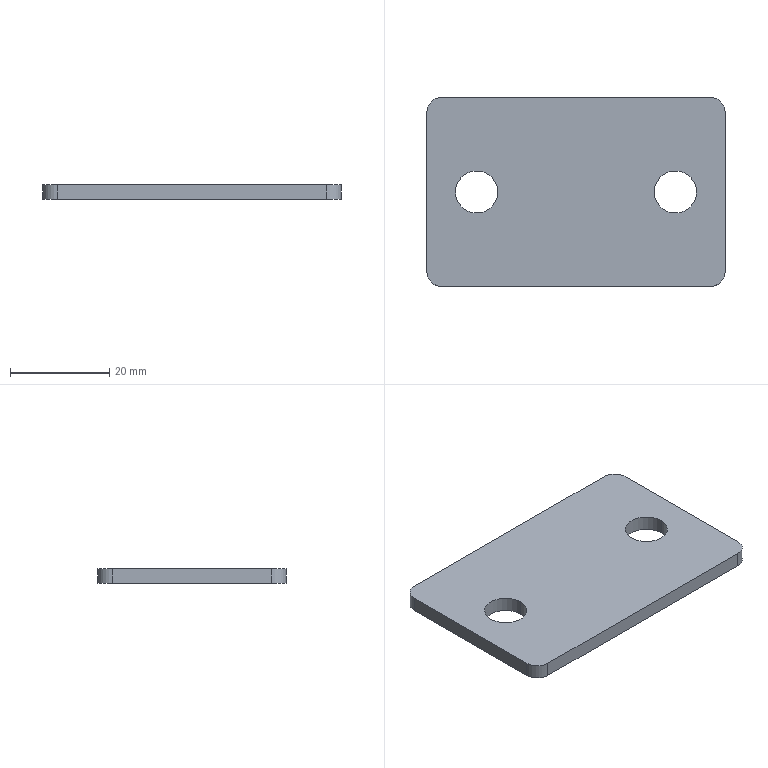Part | SolidWorks | features BaseBody 1 | 1 solid | 14 faces | box 60 x 38 x 3 mm | volume 6476 mm3 | cylinder 8 | plane 6 | commonest cylinder face diameters 6 x4 8.5 x4
STEP:
#1=CARTESIAN_POINT('',(54.25,0.,0.));
#2=VERTEX_POINT('',#1);
#3=CARTESIAN_POINT('',(45.75,0.,0.));
#4=VERTEX_POINT('',#3);
#5=CARTESIAN_POINT('',(50.,0.,0.));
#6=DIRECTION('',(0.,0.,-1.));
#7=DIRECTION('',(-1.,0.,0.));
#8=AXIS2_PLACEMENT_3D('',#5,#6,#7);
#9=CIRCLE('',#8,4.25);
#10=EDGE_CURVE('',#2,#4,#9,.T.);
#11=ORIENTED_EDGE('',*,*,#10,.F.);
#12=CARTESIAN_POINT('',(54.25,0.,-3.));
#13=VERTEX_POINT('',#12);
#14=CARTESIAN_POINT('',(54.25,0.,-3.));
#15=DIRECTION('',(0.,0.,-1.));
#16=VECTOR('',#15,1000.);
#17=LINE('',#14,#16);
#18=EDGE_CURVE('',#2,#13,#17,.T.);
#19=ORIENTED_EDGE('',*,*,#18,.T.);
#20=CARTESIAN_POINT('',(45.75,0.,-3.));
#21=VERTEX_POINT('',#20);
#22=CARTESIAN_POINT('',(50.,0.,-3.));
#23=DIRECTION('',(0.,0.,-1.));
#24=DIRECTION('',(-1.,0.,0.));
#25=AXIS2_PLACEMENT_3D('',#22,#23,#24);
#26=CIRCLE('',#25,4.25);
#27=EDGE_CURVE('',#13,#21,#26,.T.);
#28=ORIENTED_EDGE('',*,*,#27,.T.);
#29=CARTESIAN_POINT('',(45.75,0.,-3.));
#30=DIRECTION('',(0.,0.,-1.));
#31=VECTOR('',#30,1000.);
#32=LINE('',#29,#31);
#33=EDGE_CURVE('',#4,#21,#32,.T.);
#34=ORIENTED_EDGE('',*,*,#33,.F.);
#35=EDGE_LOOP('',(#11,#19,#28,#34));
#36=FACE_OUTER_BOUND('',#35,.T.);
#37=CARTESIAN_POINT('',(50.,0.,-3.));
#38=DIRECTION('',(0.,0.,-1.));
#39=DIRECTION('',(-1.,0.,0.));
#40=AXIS2_PLACEMENT_3D('',#37,#38,#39);
#41=CYLINDRICAL_SURFACE('',#40,4.25);
#42=ADVANCED_FACE('',(#36),#41,.F.);
#43=CARTESIAN_POINT('',(14.25,0.,0.));
#44=VERTEX_POINT('',#43);
#45=CARTESIAN_POINT('',(5.75,0.,0.));
#46=VERTEX_POINT('',#45);
#47=CARTESIAN_POINT('',(10.,0.,0.));
#48=DIRECTION('',(0.,0.,-1.));
#49=DIRECTION('',(-1.,0.,0.));
#50=AXIS2_PLACEMENT_3D('',#47,#48,#49);
#51=CIRCLE('',#50,4.25);
#52=EDGE_CURVE('',#44,#46,#51,.T.);
#53=ORIENTED_EDGE('',*,*,#52,.F.);
#54=CARTESIAN_POINT('',(14.25,0.,-3.));
#55=VERTEX_POINT('',#54);
#56=CARTESIAN_POINT('',(14.25,0.,-3.));
#57=DIRECTION('',(0.,0.,-1.));
#58=VECTOR('',#57,1000.);
#59=LINE('',#56,#58);
#60=EDGE_CURVE('',#44,#55,#59,.T.);
#61=ORIENTED_EDGE('',*,*,#60,.T.);
#62=CARTESIAN_POINT('',(5.75,0.,-3.));
#63=VERTEX_POINT('',#62);
#64=CARTESIAN_POINT('',(10.,0.,-3.));
#65=DIRECTION('',(0.,0.,-1.));
#66=DIRECTION('',(-1.,0.,0.));
#67=AXIS2_PLACEMENT_3D('',#64,#65,#66);
#68=CIRCLE('',#67,4.25);
#69=EDGE_CURVE('',#55,#63,#68,.T.);
#70=ORIENTED_EDGE('',*,*,#69,.T.);
#71=CARTESIAN_POINT('',(5.75,0.,-3.));
#72=DIRECTION('',(0.,0.,-1.));
#73=VECTOR('',#72,1000.);
#74=LINE('',#71,#73);
#75=EDGE_CURVE('',#46,#63,#74,.T.);
#76=ORIENTED_EDGE('',*,*,#75,.F.);
#77=EDGE_LOOP('',(#53,#61,#70,#76));
#78=FACE_OUTER_BOUND('',#77,.T.);
#79=CARTESIAN_POINT('',(10.,0.,-3.));
#80=DIRECTION('',(0.,0.,-1.));
#81=DIRECTION('',(-1.,0.,0.));
#82=AXIS2_PLACEMENT_3D('',#79,#80,#81);
#83=CYLINDRICAL_SURFACE('',#82,4.25);
#84=ADVANCED_FACE('',(#78),#83,.F.);
#85=CARTESIAN_POINT('',(57.,19.,-3.));
#86=VERTEX_POINT('',#85);
#87=CARTESIAN_POINT('',(3.,19.,-3.));
#88=VERTEX_POINT('',#87);
#89=CARTESIAN_POINT('',(3.,19.,-3.));
#90=DIRECTION('',(-1.,0.,0.));
#91=VECTOR('',#90,1000.);
#92=LINE('',#89,#91);
#93=EDGE_CURVE('',#86,#88,#92,.T.);
#94=ORIENTED_EDGE('',*,*,#93,.F.);
#95=CARTESIAN_POINT('',(60.,16.,-3.));
#96=VERTEX_POINT('',#95);
#97=CARTESIAN_POINT('',(57.,16.,-3.));
#98=DIRECTION('',(0.,0.,1.));
#99=DIRECTION('',(-1.,0.,0.));
#100=AXIS2_PLACEMENT_3D('',#97,#98,#99);
#101=CIRCLE('',#100,3.);
#102=EDGE_CURVE('',#96,#86,#101,.T.);
#103=ORIENTED_EDGE('',*,*,#102,.F.);
#104=CARTESIAN_POINT('',(60.,-16.,-3.));
#105=VERTEX_POINT('',#104);
#106=CARTESIAN_POINT('',(60.,16.,-3.));
#107=DIRECTION('',(0.,1.,0.));
#108=VECTOR('',#107,1000.);
#109=LINE('',#106,#108);
#110=EDGE_CURVE('',#105,#96,#109,.T.);
#111=ORIENTED_EDGE('',*,*,#110,.F.);
#112=CARTESIAN_POINT('',(57.,-19.,-3.));
#113=VERTEX_POINT('',#112);
#114=CARTESIAN_POINT('',(57.,-16.,-3.));
#115=DIRECTION('',(0.,0.,1.));
#116=DIRECTION('',(-1.,0.,0.));
#117=AXIS2_PLACEMENT_3D('',#114,#115,#116);
#118=CIRCLE('',#117,3.);
#119=EDGE_CURVE('',#113,#105,#118,.T.);
#120=ORIENTED_EDGE('',*,*,#119,.F.);
#121=CARTESIAN_POINT('',(3.,-19.,-3.));
#122=VERTEX_POINT('',#121);
#123=CARTESIAN_POINT('',(3.,-19.,-3.));
#124=DIRECTION('',(1.,0.,0.));
#125=VECTOR('',#124,1000.);
#126=LINE('',#123,#125);
#127=EDGE_CURVE('',#122,#113,#126,.T.);
#128=ORIENTED_EDGE('',*,*,#127,.F.);
#129=CARTESIAN_POINT('',(0.,-16.,-3.));
#130=VERTEX_POINT('',#129);
#131=CARTESIAN_POINT('',(3.,-16.,-3.));
#132=DIRECTION('',(0.,0.,1.));
#133=DIRECTION('',(-1.,0.,0.));
#134=AXIS2_PLACEMENT_3D('',#131,#132,#133);
#135=CIRCLE('',#134,3.);
#136=EDGE_CURVE('',#130,#122,#135,.T.);
#137=ORIENTED_EDGE('',*,*,#136,.F.);
#138=CARTESIAN_POINT('',(0.,16.,-3.));
#139=VERTEX_POINT('',#138);
#140=CARTESIAN_POINT('',(0.,16.,-3.));
#141=DIRECTION('',(0.,-1.,0.));
#142=VECTOR('',#141,1000.);
#143=LINE('',#140,#142);
#144=EDGE_CURVE('',#139,#130,#143,.T.);
#145=ORIENTED_EDGE('',*,*,#144,.F.);
#146=CARTESIAN_POINT('',(3.,16.,-3.));
#147=DIRECTION('',(0.,0.,1.));
#148=DIRECTION('',(-1.,0.,0.));
#149=AXIS2_PLACEMENT_3D('',#146,#147,#148);
#150=CIRCLE('',#149,3.);
#151=EDGE_CURVE('',#88,#139,#150,.T.);
#152=ORIENTED_EDGE('',*,*,#151,.F.);
#153=EDGE_LOOP('',(#94,#103,#111,#120,#128,#137,#145,#152));
#154=FACE_OUTER_BOUND('',#153,.T.);
#155=CARTESIAN_POINT('',(50.,0.,-3.));
#156=DIRECTION('',(0.,0.,-1.));
#157=DIRECTION('',(-1.,0.,0.));
#158=AXIS2_PLACEMENT_3D('',#155,#156,#157);
#159=CIRCLE('',#158,4.25);
#160=EDGE_CURVE('',#21,#13,#159,.T.);
#161=ORIENTED_EDGE('',*,*,#160,.F.);
#162=ORIENTED_EDGE('',*,*,#27,.F.);
#163=EDGE_LOOP('',(#161,#162));
#164=FACE_BOUND('',#163,.T.);
#165=CARTESIAN_POINT('',(10.,0.,-3.));
#166=DIRECTION('',(0.,0.,-1.));
#167=DIRECTION('',(-1.,0.,0.));
#168=AXIS2_PLACEMENT_3D('',#165,#166,#167);
#169=CIRCLE('',#168,4.25);
#170=EDGE_CURVE('',#63,#55,#169,.T.);
#171=ORIENTED_EDGE('',*,*,#170,.F.);
#172=ORIENTED_EDGE('',*,*,#69,.F.);
#173=EDGE_LOOP('',(#171,#172));
#174=FACE_BOUND('',#173,.T.);
#175=CARTESIAN_POINT('',(3.,16.,-3.));
#176=DIRECTION('',(0.,0.,1.));
#177=DIRECTION('',(1.,0.,0.));
#178=AXIS2_PLACEMENT_3D('',#175,#176,#177);
#179=PLANE('',#178);
#180=ADVANCED_FACE('',(#154,#164,#174),#179,.F.);
#181=ORIENTED_EDGE('',*,*,#151,.T.);
#182=CARTESIAN_POINT('',(0.,16.,0.));
#183=VERTEX_POINT('',#182);
#184=CARTESIAN_POINT('',(0.,16.,-3.));
#185=DIRECTION('',(0.,0.,1.));
#186=VECTOR('',#185,1000.);
#187=LINE('',#184,#186);
#188=EDGE_CURVE('',#139,#183,#187,.T.);
#189=ORIENTED_EDGE('',*,*,#188,.T.);
#190=CARTESIAN_POINT('',(3.,19.,0.));
#191=VERTEX_POINT('',#190);
#192=CARTESIAN_POINT('',(3.,16.,0.));
#193=DIRECTION('',(0.,0.,-1.));
#194=DIRECTION('',(-1.,0.,0.));
#195=AXIS2_PLACEMENT_3D('',#192,#193,#194);
#196=CIRCLE('',#195,3.);
#197=EDGE_CURVE('',#183,#191,#196,.T.);
#198=ORIENTED_EDGE('',*,*,#197,.T.);
#199=CARTESIAN_POINT('',(3.,19.,-3.));
#200=DIRECTION('',(0.,0.,-1.));
#201=VECTOR('',#200,1000.);
#202=LINE('',#199,#201);
#203=EDGE_CURVE('',#191,#88,#202,.T.);
#204=ORIENTED_EDGE('',*,*,#203,.T.);
#205=EDGE_LOOP('',(#181,#189,#198,#204));
#206=FACE_OUTER_BOUND('',#205,.T.);
#207=CARTESIAN_POINT('',(3.,16.,-3.));
#208=DIRECTION('',(0.,0.,-1.));
#209=DIRECTION('',(-1.,0.,0.));
#210=AXIS2_PLACEMENT_3D('',#207,#208,#209);
#211=CYLINDRICAL_SURFACE('',#210,3.);
#212=ADVANCED_FACE('',(#206),#211,.T.);
#213=ORIENTED_EDGE('',*,*,#93,.T.);
#214=ORIENTED_EDGE('',*,*,#203,.F.);
#215=CARTESIAN_POINT('',(57.,19.,0.));
#216=VERTEX_POINT('',#215);
#217=CARTESIAN_POINT('',(57.,19.,0.));
#218=DIRECTION('',(1.,0.,0.));
#219=VECTOR('',#218,1000.);
#220=LINE('',#217,#219);
#221=EDGE_CURVE('',#191,#216,#220,.T.);
#222=ORIENTED_EDGE('',*,*,#221,.T.);
#223=CARTESIAN_POINT('',(57.,19.,-3.));
#224=DIRECTION('',(0.,0.,-1.));
#225=VECTOR('',#224,1000.);
#226=LINE('',#223,#225);
#227=EDGE_CURVE('',#216,#86,#226,.T.);
#228=ORIENTED_EDGE('',*,*,#227,.T.);
#229=EDGE_LOOP('',(#213,#214,#222,#228));
#230=FACE_OUTER_BOUND('',#229,.T.);
#231=CARTESIAN_POINT('',(57.,19.,-3.));
#232=DIRECTION('',(0.,1.,0.));
#233=DIRECTION('',(0.,0.,1.));
#234=AXIS2_PLACEMENT_3D('',#231,#232,#233);
#235=PLANE('',#234);
#236=ADVANCED_FACE('',(#230),#235,.T.);
#237=ORIENTED_EDGE('',*,*,#102,.T.);
#238=ORIENTED_EDGE('',*,*,#227,.F.);
#239=CARTESIAN_POINT('',(60.,16.,0.));
#240=VERTEX_POINT('',#239);
#241=CARTESIAN_POINT('',(57.,16.,0.));
#242=DIRECTION('',(0.,0.,-1.));
#243=DIRECTION('',(-1.,0.,0.));
#244=AXIS2_PLACEMENT_3D('',#241,#242,#243);
#245=CIRCLE('',#244,3.);
#246=EDGE_CURVE('',#216,#240,#245,.T.);
#247=ORIENTED_EDGE('',*,*,#246,.T.);
#248=CARTESIAN_POINT('',(60.,16.,-3.));
#249=DIRECTION('',(0.,0.,-1.));
#250=VECTOR('',#249,1000.);
#251=LINE('',#248,#250);
#252=EDGE_CURVE('',#240,#96,#251,.T.);
#253=ORIENTED_EDGE('',*,*,#252,.T.);
#254=EDGE_LOOP('',(#237,#238,#247,#253));
#255=FACE_OUTER_BOUND('',#254,.T.);
#256=CARTESIAN_POINT('',(57.,16.,-3.));
#257=DIRECTION('',(0.,0.,-1.));
#258=DIRECTION('',(-1.,0.,0.));
#259=AXIS2_PLACEMENT_3D('',#256,#257,#258);
#260=CYLINDRICAL_SURFACE('',#259,3.);
#261=ADVANCED_FACE('',(#255),#260,.T.);
#262=ORIENTED_EDGE('',*,*,#110,.T.);
#263=ORIENTED_EDGE('',*,*,#252,.F.);
#264=CARTESIAN_POINT('',(60.,-16.,0.));
#265=VERTEX_POINT('',#264);
#266=CARTESIAN_POINT('',(60.,-16.,0.));
#267=DIRECTION('',(0.,-1.,0.));
#268=VECTOR('',#267,1000.);
#269=LINE('',#266,#268);
#270=EDGE_CURVE('',#240,#265,#269,.T.);
#271=ORIENTED_EDGE('',*,*,#270,.T.);
#272=CARTESIAN_POINT('',(60.,-16.,-3.));
#273=DIRECTION('',(0.,0.,-1.));
#274=VECTOR('',#273,1000.);
#275=LINE('',#272,#274);
#276=EDGE_CURVE('',#265,#105,#275,.T.);
#277=ORIENTED_EDGE('',*,*,#276,.T.);
#278=EDGE_LOOP('',(#262,#263,#271,#277));
#279=FACE_OUTER_BOUND('',#278,.T.);
#280=CARTESIAN_POINT('',(60.,-16.,-3.));
#281=DIRECTION('',(1.,0.,0.));
#282=DIRECTION('',(0.,0.,-1.));
#283=AXIS2_PLACEMENT_3D('',#280,#281,#282);
#284=PLANE('',#283);
#285=ADVANCED_FACE('',(#279),#284,.T.);
#286=ORIENTED_EDGE('',*,*,#119,.T.);
#287=ORIENTED_EDGE('',*,*,#276,.F.);
#288=CARTESIAN_POINT('',(57.,-19.,0.));
#289=VERTEX_POINT('',#288);
#290=CARTESIAN_POINT('',(57.,-16.,0.));
#291=DIRECTION('',(0.,0.,-1.));
#292=DIRECTION('',(-1.,0.,0.));
#293=AXIS2_PLACEMENT_3D('',#290,#291,#292);
#294=CIRCLE('',#293,3.);
#295=EDGE_CURVE('',#265,#289,#294,.T.);
#296=ORIENTED_EDGE('',*,*,#295,.T.);
#297=CARTESIAN_POINT('',(57.,-19.,-3.));
#298=DIRECTION('',(0.,0.,-1.));
#299=VECTOR('',#298,1000.);
#300=LINE('',#297,#299);
#301=EDGE_CURVE('',#289,#113,#300,.T.);
#302=ORIENTED_EDGE('',*,*,#301,.T.);
#303=EDGE_LOOP('',(#286,#287,#296,#302));
#304=FACE_OUTER_BOUND('',#303,.T.);
#305=CARTESIAN_POINT('',(57.,-16.,-3.));
#306=DIRECTION('',(0.,0.,-1.));
#307=DIRECTION('',(-1.,0.,0.));
#308=AXIS2_PLACEMENT_3D('',#305,#306,#307);
#309=CYLINDRICAL_SURFACE('',#308,3.);
#310=ADVANCED_FACE('',(#304),#309,.T.);
#311=ORIENTED_EDGE('',*,*,#127,.T.);
#312=ORIENTED_EDGE('',*,*,#301,.F.);
#313=CARTESIAN_POINT('',(3.,-19.,0.));
#314=VERTEX_POINT('',#313);
#315=CARTESIAN_POINT('',(3.,-19.,0.));
#316=DIRECTION('',(-1.,0.,0.));
#317=VECTOR('',#316,1000.);
#318=LINE('',#315,#317);
#319=EDGE_CURVE('',#289,#314,#318,.T.);
#320=ORIENTED_EDGE('',*,*,#319,.T.);
#321=CARTESIAN_POINT('',(3.,-19.,-3.));
#322=DIRECTION('',(0.,0.,-1.));
#323=VECTOR('',#322,1000.);
#324=LINE('',#321,#323);
#325=EDGE_CURVE('',#314,#122,#324,.T.);
#326=ORIENTED_EDGE('',*,*,#325,.T.);
#327=EDGE_LOOP('',(#311,#312,#320,#326));
#328=FACE_OUTER_BOUND('',#327,.T.);
#329=CARTESIAN_POINT('',(3.,-19.,-3.));
#330=DIRECTION('',(0.,-1.,0.));
#331=DIRECTION('',(0.,0.,-1.));
#332=AXIS2_PLACEMENT_3D('',#329,#330,#331);
#333=PLANE('',#332);
#334=ADVANCED_FACE('',(#328),#333,.T.);
#335=ORIENTED_EDGE('',*,*,#136,.T.);
#336=ORIENTED_EDGE('',*,*,#325,.F.);
#337=CARTESIAN_POINT('',(0.,-16.,0.));
#338=VERTEX_POINT('',#337);
#339=CARTESIAN_POINT('',(3.,-16.,0.));
#340=DIRECTION('',(0.,0.,-1.));
#341=DIRECTION('',(-1.,0.,0.));
#342=AXIS2_PLACEMENT_3D('',#339,#340,#341);
#343=CIRCLE('',#342,3.);
#344=EDGE_CURVE('',#314,#338,#343,.T.);
#345=ORIENTED_EDGE('',*,*,#344,.T.);
#346=CARTESIAN_POINT('',(0.,-16.,-3.));
#347=DIRECTION('',(0.,0.,-1.));
#348=VECTOR('',#347,1000.);
#349=LINE('',#346,#348);
#350=EDGE_CURVE('',#338,#130,#349,.T.);
#351=ORIENTED_EDGE('',*,*,#350,.T.);
#352=EDGE_LOOP('',(#335,#336,#345,#351));
#353=FACE_OUTER_BOUND('',#352,.T.);
#354=CARTESIAN_POINT('',(3.,-16.,-3.));
#355=DIRECTION('',(0.,0.,-1.));
#356=DIRECTION('',(-1.,0.,0.));
#357=AXIS2_PLACEMENT_3D('',#354,#355,#356);
#358=CYLINDRICAL_SURFACE('',#357,3.);
#359=ADVANCED_FACE('',(#353),#358,.T.);
#360=ORIENTED_EDGE('',*,*,#144,.T.);
#361=ORIENTED_EDGE('',*,*,#350,.F.);
#362=CARTESIAN_POINT('',(0.,16.,0.));
#363=DIRECTION('',(0.,1.,0.));
#364=VECTOR('',#363,1000.);
#365=LINE('',#362,#364);
#366=EDGE_CURVE('',#338,#183,#365,.T.);
#367=ORIENTED_EDGE('',*,*,#366,.T.);
#368=ORIENTED_EDGE('',*,*,#188,.F.);
#369=EDGE_LOOP('',(#360,#361,#367,#368));
#370=FACE_OUTER_BOUND('',#369,.T.);
#371=CARTESIAN_POINT('',(0.,16.,-3.));
#372=DIRECTION('',(-1.,0.,0.));
#373=DIRECTION('',(0.,0.,1.));
#374=AXIS2_PLACEMENT_3D('',#371,#372,#373);
#375=PLANE('',#374);
#376=ADVANCED_FACE('',(#370),#375,.T.);
#377=ORIENTED_EDGE('',*,*,#18,.F.);
#378=CARTESIAN_POINT('',(50.,0.,0.));
#379=DIRECTION('',(0.,0.,-1.));
#380=DIRECTION('',(-1.,0.,0.));
#381=AXIS2_PLACEMENT_3D('',#378,#379,#380);
#382=CIRCLE('',#381,4.25);
#383=EDGE_CURVE('',#4,#2,#382,.T.);
#384=ORIENTED_EDGE('',*,*,#383,.F.);
#385=ORIENTED_EDGE('',*,*,#33,.T.);
#386=ORIENTED_EDGE('',*,*,#160,.T.);
#387=EDGE_LOOP('',(#377,#384,#385,#386));
#388=FACE_OUTER_BOUND('',#387,.T.);
#389=CARTESIAN_POINT('',(50.,0.,-3.));
#390=DIRECTION('',(0.,0.,-1.));
#391=DIRECTION('',(-1.,0.,0.));
#392=AXIS2_PLACEMENT_3D('',#389,#390,#391);
#393=CYLINDRICAL_SURFACE('',#392,4.25);
#394=ADVANCED_FACE('',(#388),#393,.F.);
#395=ORIENTED_EDGE('',*,*,#60,.F.);
#396=CARTESIAN_POINT('',(10.,0.,0.));
#397=DIRECTION('',(0.,0.,-1.));
#398=DIRECTION('',(-1.,0.,0.));
#399=AXIS2_PLACEMENT_3D('',#396,#397,#398);
#400=CIRCLE('',#399,4.25);
#401=EDGE_CURVE('',#46,#44,#400,.T.);
#402=ORIENTED_EDGE('',*,*,#401,.F.);
#403=ORIENTED_EDGE('',*,*,#75,.T.);
#404=ORIENTED_EDGE('',*,*,#170,.T.);
#405=EDGE_LOOP('',(#395,#402,#403,#404));
#406=FACE_OUTER_BOUND('',#405,.T.);
#407=CARTESIAN_POINT('',(10.,0.,-3.));
#408=DIRECTION('',(0.,0.,-1.));
#409=DIRECTION('',(-1.,0.,0.));
#410=AXIS2_PLACEMENT_3D('',#407,#408,#409);
#411=CYLINDRICAL_SURFACE('',#410,4.25);
#412=ADVANCED_FACE('',(#406),#411,.F.);
#413=ORIENTED_EDGE('',*,*,#246,.F.);
#414=ORIENTED_EDGE('',*,*,#221,.F.);
#415=ORIENTED_EDGE('',*,*,#197,.F.);
#416=ORIENTED_EDGE('',*,*,#366,.F.);
#417=ORIENTED_EDGE('',*,*,#344,.F.);
#418=ORIENTED_EDGE('',*,*,#319,.F.);
#419=ORIENTED_EDGE('',*,*,#295,.F.);
#420=ORIENTED_EDGE('',*,*,#270,.F.);
#421=EDGE_LOOP('',(#413,#414,#415,#416,#417,#418,#419,#420));
#422=FACE_OUTER_BOUND('',#421,.T.);
#423=ORIENTED_EDGE('',*,*,#383,.T.);
#424=ORIENTED_EDGE('',*,*,#10,.T.);
#425=EDGE_LOOP('',(#423,#424));
#426=FACE_BOUND('',#425,.T.);
#427=ORIENTED_EDGE('',*,*,#401,.T.);
#428=ORIENTED_EDGE('',*,*,#52,.T.);
#429=EDGE_LOOP('',(#427,#428));
#430=FACE_BOUND('',#429,.T.);
#431=CARTESIAN_POINT('',(3.,16.,0.));
#432=DIRECTION('',(0.,0.,1.));
#433=DIRECTION('',(1.,0.,0.));
#434=AXIS2_PLACEMENT_3D('',#431,#432,#433);
#435=PLANE('',#434);
#436=ADVANCED_FACE('',(#422,#426,#430),#435,.T.);
#437=CLOSED_SHELL('',(#42,#84,#180,#212,#236,#261,#285,#310,#334,#359,#376,#394,#412,#436));
#438=MANIFOLD_SOLID_BREP('',#437);
#439=CARTESIAN_POINT('',(0.,0.,0.));
#440=DIRECTION('',(0.,0.,1.));
#441=DIRECTION('',(1.,0.,0.));
#442=AXIS2_PLACEMENT_3D('',#439,#440,#441);
#443=(LENGTH_UNIT()NAMED_UNIT(*)SI_UNIT(.MILLI.,.METRE.));
#444=UNCERTAINTY_MEASURE_WITH_UNIT(LENGTH_MEASURE(0.00001),#443,'','');
#445=(NAMED_UNIT(*)PLANE_ANGLE_UNIT()SI_UNIT($,.RADIAN.));
#446=(NAMED_UNIT(*)SI_UNIT($,.STERADIAN.)SOLID_ANGLE_UNIT());
#447=(GEOMETRIC_REPRESENTATION_CONTEXT(3)GLOBAL_UNCERTAINTY_ASSIGNED_CONTEXT((#444))GLOBAL_UNIT_ASSIGNED_CONTEXT((#443,#445,#446))REPRESENTATION_CONTEXT('',''));
#448=ADVANCED_BREP_SHAPE_REPRESENTATION('',(#438,#442),#447);